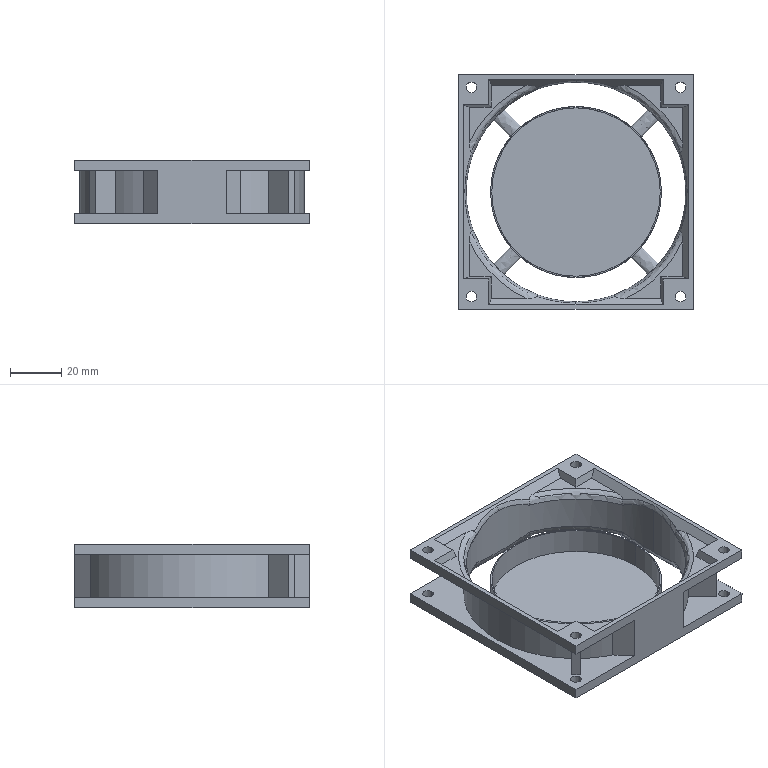Part | STEP file | SRQ-FSK | 1 solid | 128 faces | box 92 x 92 x 25 mm | volume 27792 mm3 | plane 68 | spline 32 | cylinder 28 | commonest cylinder face diameters 4.2 x16 88 x6 66 x2 67 x2 86 x2